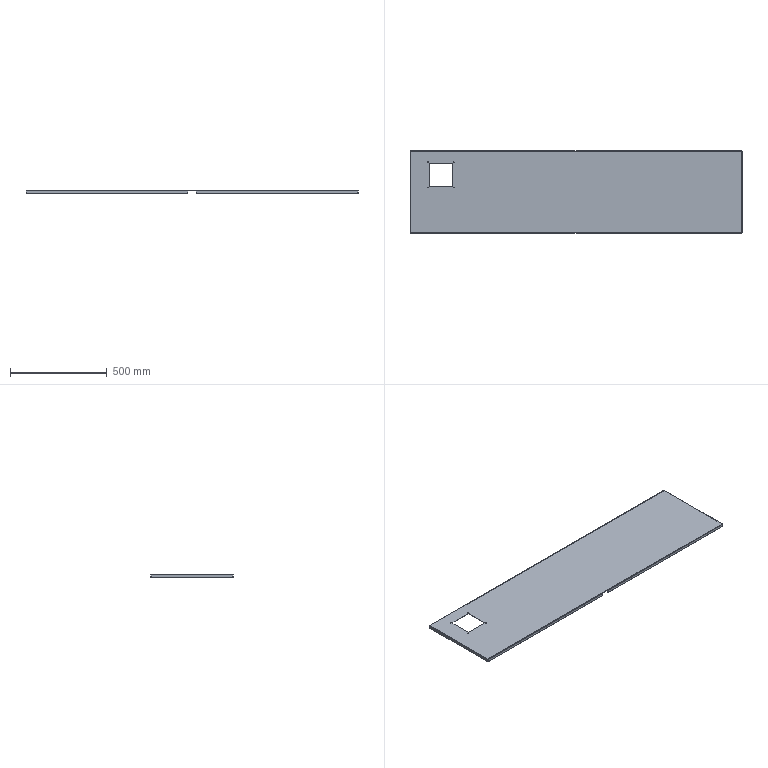Part | STEP file | 1 solid | 62 faces | box 1718 x 428 x 15 mm | volume 1162465 mm3 | plane 36 | cylinder 18 | spline 8 | commonest cylinder face diameters 4.5 x8 1 x6 4 x4